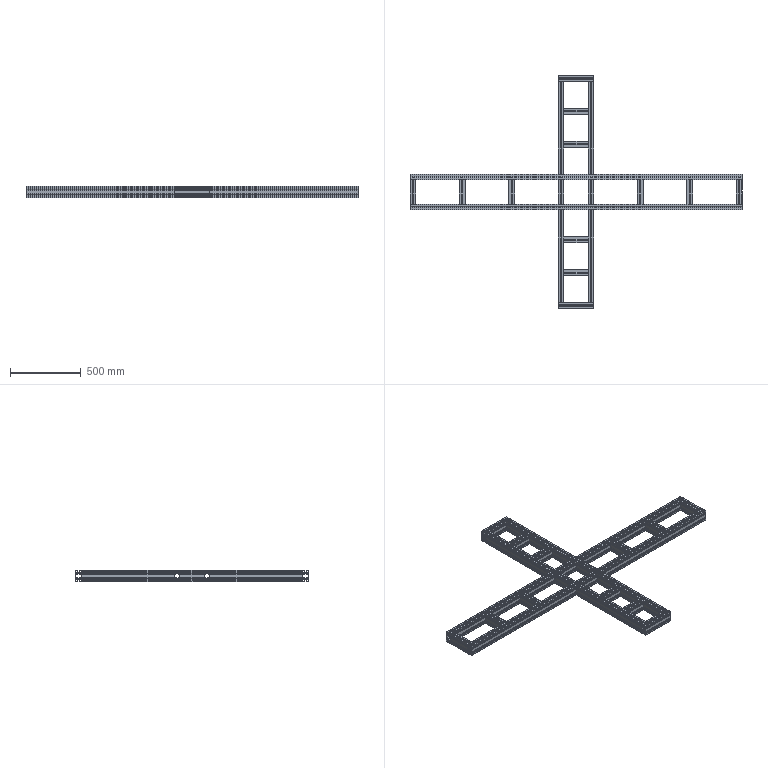Part | SolidWorks | features WeldMemberFeat 1, WeldmentFeature 1 | 20 solids | 5384 faces | volume 6888889 mm3 | plane 4920 | cylinder 464 | commonest cylinder face diameters 9.6 x344 6.6 x80 0.6 x40